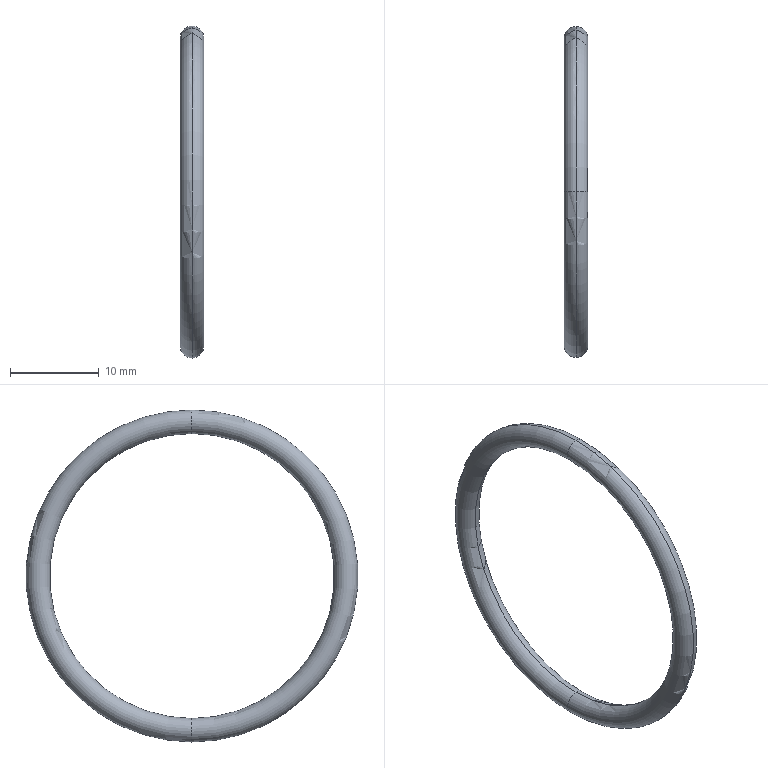Part | SolidWorks | features Revolution 1 | 1 solid | 4 faces | box 2.65 x 37.35 x 37.35 mm | volume 601.258 mm3 | torus 4
STEP:
#1=CARTESIAN_POINT('',(5.,0.,-18.675));
#2=VERTEX_POINT('',#1);
#3=CARTESIAN_POINT('',(5.,0.,-16.025));
#4=VERTEX_POINT('',#3);
#5=CARTESIAN_POINT('',(5.,0.,-17.35));
#6=DIRECTION('',(0.,1.,0.));
#7=DIRECTION('',(0.,0.,1.));
#8=AXIS2_PLACEMENT_3D('',#5,#6,#7);
#9=CIRCLE('',#8,1.325);
#10=EDGE_CURVE('',#2,#4,#9,.T.);
#11=ORIENTED_EDGE('',*,*,#10,.F.);
#12=CARTESIAN_POINT('',(5.,0.,18.675));
#13=VERTEX_POINT('',#12);
#14=CARTESIAN_POINT('',(5.,0.,0.));
#15=DIRECTION('',(-1.,0.,0.));
#16=DIRECTION('',(0.,0.,1.));
#17=AXIS2_PLACEMENT_3D('',#14,#15,#16);
#18=CIRCLE('',#17,18.675);
#19=EDGE_CURVE('',#2,#13,#18,.T.);
#20=ORIENTED_EDGE('',*,*,#19,.T.);
#21=CARTESIAN_POINT('',(5.,0.,16.025));
#22=VERTEX_POINT('',#21);
#23=CARTESIAN_POINT('',(5.,0.,17.35));
#24=DIRECTION('',(0.,-1.,0.));
#25=DIRECTION('',(0.,0.,-1.));
#26=AXIS2_PLACEMENT_3D('',#23,#24,#25);
#27=CIRCLE('',#26,1.325);
#28=EDGE_CURVE('',#13,#22,#27,.T.);
#29=ORIENTED_EDGE('',*,*,#28,.T.);
#30=CARTESIAN_POINT('',(5.,0.,0.));
#31=DIRECTION('',(-1.,0.,0.));
#32=DIRECTION('',(0.,0.,1.));
#33=AXIS2_PLACEMENT_3D('',#30,#31,#32);
#34=CIRCLE('',#33,16.025);
#35=EDGE_CURVE('',#4,#22,#34,.T.);
#36=ORIENTED_EDGE('',*,*,#35,.F.);
#37=EDGE_LOOP('',(#11,#20,#29,#36));
#38=FACE_OUTER_BOUND('',#37,.T.);
#39=CARTESIAN_POINT('',(5.,0.,0.));
#40=DIRECTION('',(-1.,0.,0.));
#41=DIRECTION('',(0.,0.,1.));
#42=AXIS2_PLACEMENT_3D('',#39,#40,#41);
#43=TOROIDAL_SURFACE('',#42,17.35,1.325);
#44=ADVANCED_FACE('',(#38),#43,.T.);
#45=ORIENTED_EDGE('',*,*,#28,.F.);
#46=CARTESIAN_POINT('',(5.,0.,0.));
#47=DIRECTION('',(-1.,0.,0.));
#48=DIRECTION('',(0.,0.,1.));
#49=AXIS2_PLACEMENT_3D('',#46,#47,#48);
#50=CIRCLE('',#49,18.675);
#51=EDGE_CURVE('',#13,#2,#50,.T.);
#52=ORIENTED_EDGE('',*,*,#51,.T.);
#53=ORIENTED_EDGE('',*,*,#10,.T.);
#54=CARTESIAN_POINT('',(5.,0.,0.));
#55=DIRECTION('',(-1.,0.,0.));
#56=DIRECTION('',(0.,0.,1.));
#57=AXIS2_PLACEMENT_3D('',#54,#55,#56);
#58=CIRCLE('',#57,16.025);
#59=EDGE_CURVE('',#22,#4,#58,.T.);
#60=ORIENTED_EDGE('',*,*,#59,.F.);
#61=EDGE_LOOP('',(#45,#52,#53,#60));
#62=FACE_OUTER_BOUND('',#61,.T.);
#63=CARTESIAN_POINT('',(5.,0.,0.));
#64=DIRECTION('',(-1.,0.,0.));
#65=DIRECTION('',(0.,0.,1.));
#66=AXIS2_PLACEMENT_3D('',#63,#64,#65);
#67=TOROIDAL_SURFACE('',#66,17.35,1.325);
#68=ADVANCED_FACE('',(#62),#67,.T.);
#69=ORIENTED_EDGE('',*,*,#51,.F.);
#70=CARTESIAN_POINT('',(5.,0.,17.35));
#71=DIRECTION('',(0.,-1.,0.));
#72=DIRECTION('',(0.,0.,-1.));
#73=AXIS2_PLACEMENT_3D('',#70,#71,#72);
#74=CIRCLE('',#73,1.325);
#75=EDGE_CURVE('',#22,#13,#74,.T.);
#76=ORIENTED_EDGE('',*,*,#75,.F.);
#77=ORIENTED_EDGE('',*,*,#59,.T.);
#78=CARTESIAN_POINT('',(5.,0.,-17.35));
#79=DIRECTION('',(0.,1.,0.));
#80=DIRECTION('',(0.,0.,1.));
#81=AXIS2_PLACEMENT_3D('',#78,#79,#80);
#82=CIRCLE('',#81,1.325);
#83=EDGE_CURVE('',#4,#2,#82,.T.);
#84=ORIENTED_EDGE('',*,*,#83,.T.);
#85=EDGE_LOOP('',(#69,#76,#77,#84));
#86=FACE_OUTER_BOUND('',#85,.T.);
#87=CARTESIAN_POINT('',(5.,0.,0.));
#88=DIRECTION('',(-1.,0.,0.));
#89=DIRECTION('',(0.,0.,1.));
#90=AXIS2_PLACEMENT_3D('',#87,#88,#89);
#91=TOROIDAL_SURFACE('',#90,17.35,1.325);
#92=ADVANCED_FACE('',(#86),#91,.T.);
#93=ORIENTED_EDGE('',*,*,#19,.F.);
#94=ORIENTED_EDGE('',*,*,#83,.F.);
#95=ORIENTED_EDGE('',*,*,#35,.T.);
#96=ORIENTED_EDGE('',*,*,#75,.T.);
#97=EDGE_LOOP('',(#93,#94,#95,#96));
#98=FACE_OUTER_BOUND('',#97,.T.);
#99=CARTESIAN_POINT('',(5.,0.,0.));
#100=DIRECTION('',(-1.,0.,0.));
#101=DIRECTION('',(0.,0.,1.));
#102=AXIS2_PLACEMENT_3D('',#99,#100,#101);
#103=TOROIDAL_SURFACE('',#102,17.35,1.325);
#104=ADVANCED_FACE('',(#98),#103,.T.);
#105=CLOSED_SHELL('',(#44,#68,#92,#104));
#106=MANIFOLD_SOLID_BREP('',#105);
#107=CARTESIAN_POINT('',(0.,0.,0.));
#108=DIRECTION('',(0.,0.,1.));
#109=DIRECTION('',(1.,0.,0.));
#110=AXIS2_PLACEMENT_3D('',#107,#108,#109);
#111=(LENGTH_UNIT()NAMED_UNIT(*)SI_UNIT(.MILLI.,.METRE.));
#112=UNCERTAINTY_MEASURE_WITH_UNIT(LENGTH_MEASURE(0.00001),#111,'','');
#113=(NAMED_UNIT(*)PLANE_ANGLE_UNIT()SI_UNIT($,.RADIAN.));
#114=(NAMED_UNIT(*)SI_UNIT($,.STERADIAN.)SOLID_ANGLE_UNIT());
#115=(GEOMETRIC_REPRESENTATION_CONTEXT(3)GLOBAL_UNCERTAINTY_ASSIGNED_CONTEXT((#112))GLOBAL_UNIT_ASSIGNED_CONTEXT((#111,#113,#114))REPRESENTATION_CONTEXT('',''));
#116=ADVANCED_BREP_SHAPE_REPRESENTATION('',(#106,#110),#115);